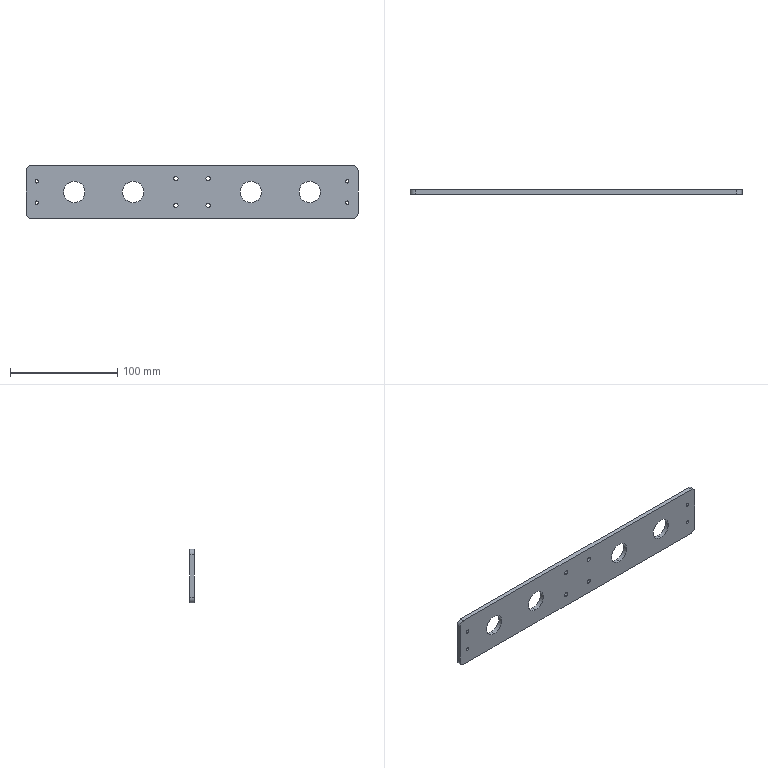Part | SolidWorks | features BaseBody 1 | 1 solid | 34 faces | box 310 x 4 x 50 mm | volume 56558 mm3 | cylinder 28 | plane 6 | commonest cylinder face diameters 3.2 x8 4 x8 20 x8 10 x4
STEP:
#1=CARTESIAN_POINT('',(15.,4.,-10.5));
#2=VERTEX_POINT('',#1);
#3=CARTESIAN_POINT('',(15.,4.,-14.5));
#4=VERTEX_POINT('',#3);
#5=CARTESIAN_POINT('',(15.,4.,-12.5));
#6=DIRECTION('',(0.,-1.,0.));
#7=DIRECTION('',(0.,0.,-1.));
#8=AXIS2_PLACEMENT_3D('',#5,#6,#7);
#9=CIRCLE('',#8,2.);
#10=EDGE_CURVE('',#2,#4,#9,.T.);
#11=ORIENTED_EDGE('',*,*,#10,.F.);
#12=CARTESIAN_POINT('',(15.,0.,-10.5));
#13=VERTEX_POINT('',#12);
#14=CARTESIAN_POINT('',(15.,4.,-10.5));
#15=DIRECTION('',(0.,-1.,0.));
#16=VECTOR('',#15,1000.);
#17=LINE('',#14,#16);
#18=EDGE_CURVE('',#2,#13,#17,.T.);
#19=ORIENTED_EDGE('',*,*,#18,.T.);
#20=CARTESIAN_POINT('',(15.,0.,-14.5));
#21=VERTEX_POINT('',#20);
#22=CARTESIAN_POINT('',(15.,0.,-12.5));
#23=DIRECTION('',(0.,-1.,0.));
#24=DIRECTION('',(0.,0.,-1.));
#25=AXIS2_PLACEMENT_3D('',#22,#23,#24);
#26=CIRCLE('',#25,2.);
#27=EDGE_CURVE('',#13,#21,#26,.T.);
#28=ORIENTED_EDGE('',*,*,#27,.T.);
#29=CARTESIAN_POINT('',(15.,4.,-14.5));
#30=DIRECTION('',(0.,-1.,0.));
#31=VECTOR('',#30,1000.);
#32=LINE('',#29,#31);
#33=EDGE_CURVE('',#4,#21,#32,.T.);
#34=ORIENTED_EDGE('',*,*,#33,.F.);
#35=EDGE_LOOP('',(#11,#19,#28,#34));
#36=FACE_OUTER_BOUND('',#35,.T.);
#37=CARTESIAN_POINT('',(15.,4.,-12.5));
#38=DIRECTION('',(0.,-1.,0.));
#39=DIRECTION('',(0.,0.,-1.));
#40=AXIS2_PLACEMENT_3D('',#37,#38,#39);
#41=CYLINDRICAL_SURFACE('',#40,2.);
#42=ADVANCED_FACE('',(#36),#41,.F.);
#43=CARTESIAN_POINT('',(15.,4.,14.5));
#44=VERTEX_POINT('',#43);
#45=CARTESIAN_POINT('',(15.,4.,10.5));
#46=VERTEX_POINT('',#45);
#47=CARTESIAN_POINT('',(15.,4.,12.5));
#48=DIRECTION('',(0.,-1.,0.));
#49=DIRECTION('',(0.,0.,-1.));
#50=AXIS2_PLACEMENT_3D('',#47,#48,#49);
#51=CIRCLE('',#50,2.);
#52=EDGE_CURVE('',#44,#46,#51,.T.);
#53=ORIENTED_EDGE('',*,*,#52,.F.);
#54=CARTESIAN_POINT('',(15.,0.,14.5));
#55=VERTEX_POINT('',#54);
#56=CARTESIAN_POINT('',(15.,4.,14.5));
#57=DIRECTION('',(0.,-1.,0.));
#58=VECTOR('',#57,1000.);
#59=LINE('',#56,#58);
#60=EDGE_CURVE('',#44,#55,#59,.T.);
#61=ORIENTED_EDGE('',*,*,#60,.T.);
#62=CARTESIAN_POINT('',(15.,0.,10.5));
#63=VERTEX_POINT('',#62);
#64=CARTESIAN_POINT('',(15.,0.,12.5));
#65=DIRECTION('',(0.,-1.,0.));
#66=DIRECTION('',(0.,0.,-1.));
#67=AXIS2_PLACEMENT_3D('',#64,#65,#66);
#68=CIRCLE('',#67,2.);
#69=EDGE_CURVE('',#55,#63,#68,.T.);
#70=ORIENTED_EDGE('',*,*,#69,.T.);
#71=CARTESIAN_POINT('',(15.,4.,10.5));
#72=DIRECTION('',(0.,-1.,0.));
#73=VECTOR('',#72,1000.);
#74=LINE('',#71,#73);
#75=EDGE_CURVE('',#46,#63,#74,.T.);
#76=ORIENTED_EDGE('',*,*,#75,.F.);
#77=EDGE_LOOP('',(#53,#61,#70,#76));
#78=FACE_OUTER_BOUND('',#77,.T.);
#79=CARTESIAN_POINT('',(15.,4.,12.5));
#80=DIRECTION('',(0.,-1.,0.));
#81=DIRECTION('',(0.,0.,-1.));
#82=AXIS2_PLACEMENT_3D('',#79,#80,#81);
#83=CYLINDRICAL_SURFACE('',#82,2.);
#84=ADVANCED_FACE('',(#78),#83,.F.);
#85=CARTESIAN_POINT('',(-15.,4.,14.5));
#86=VERTEX_POINT('',#85);
#87=CARTESIAN_POINT('',(-15.,4.,10.5));
#88=VERTEX_POINT('',#87);
#89=CARTESIAN_POINT('',(-15.,4.,12.5));
#90=DIRECTION('',(0.,-1.,0.));
#91=DIRECTION('',(0.,0.,-1.));
#92=AXIS2_PLACEMENT_3D('',#89,#90,#91);
#93=CIRCLE('',#92,2.);
#94=EDGE_CURVE('',#86,#88,#93,.T.);
#95=ORIENTED_EDGE('',*,*,#94,.F.);
#96=CARTESIAN_POINT('',(-15.,0.,14.5));
#97=VERTEX_POINT('',#96);
#98=CARTESIAN_POINT('',(-15.,4.,14.5));
#99=DIRECTION('',(0.,-1.,0.));
#100=VECTOR('',#99,1000.);
#101=LINE('',#98,#100);
#102=EDGE_CURVE('',#86,#97,#101,.T.);
#103=ORIENTED_EDGE('',*,*,#102,.T.);
#104=CARTESIAN_POINT('',(-15.,0.,10.5));
#105=VERTEX_POINT('',#104);
#106=CARTESIAN_POINT('',(-15.,0.,12.5));
#107=DIRECTION('',(0.,-1.,0.));
#108=DIRECTION('',(0.,0.,-1.));
#109=AXIS2_PLACEMENT_3D('',#106,#107,#108);
#110=CIRCLE('',#109,2.);
#111=EDGE_CURVE('',#97,#105,#110,.T.);
#112=ORIENTED_EDGE('',*,*,#111,.T.);
#113=CARTESIAN_POINT('',(-15.,4.,10.5));
#114=DIRECTION('',(0.,-1.,0.));
#115=VECTOR('',#114,1000.);
#116=LINE('',#113,#115);
#117=EDGE_CURVE('',#88,#105,#116,.T.);
#118=ORIENTED_EDGE('',*,*,#117,.F.);
#119=EDGE_LOOP('',(#95,#103,#112,#118));
#120=FACE_OUTER_BOUND('',#119,.T.);
#121=CARTESIAN_POINT('',(-15.,4.,12.5));
#122=DIRECTION('',(0.,-1.,0.));
#123=DIRECTION('',(0.,0.,-1.));
#124=AXIS2_PLACEMENT_3D('',#121,#122,#123);
#125=CYLINDRICAL_SURFACE('',#124,2.);
#126=ADVANCED_FACE('',(#120),#125,.F.);
#127=CARTESIAN_POINT('',(-15.,4.,-10.5));
#128=VERTEX_POINT('',#127);
#129=CARTESIAN_POINT('',(-15.,4.,-14.5));
#130=VERTEX_POINT('',#129);
#131=CARTESIAN_POINT('',(-15.,4.,-12.5));
#132=DIRECTION('',(0.,-1.,0.));
#133=DIRECTION('',(0.,0.,-1.));
#134=AXIS2_PLACEMENT_3D('',#131,#132,#133);
#135=CIRCLE('',#134,2.);
#136=EDGE_CURVE('',#128,#130,#135,.T.);
#137=ORIENTED_EDGE('',*,*,#136,.F.);
#138=CARTESIAN_POINT('',(-15.,0.,-10.5));
#139=VERTEX_POINT('',#138);
#140=CARTESIAN_POINT('',(-15.,4.,-10.5));
#141=DIRECTION('',(0.,-1.,0.));
#142=VECTOR('',#141,1000.);
#143=LINE('',#140,#142);
#144=EDGE_CURVE('',#128,#139,#143,.T.);
#145=ORIENTED_EDGE('',*,*,#144,.T.);
#146=CARTESIAN_POINT('',(-15.,0.,-14.5));
#147=VERTEX_POINT('',#146);
#148=CARTESIAN_POINT('',(-15.,0.,-12.5));
#149=DIRECTION('',(0.,-1.,0.));
#150=DIRECTION('',(0.,0.,-1.));
#151=AXIS2_PLACEMENT_3D('',#148,#149,#150);
#152=CIRCLE('',#151,2.);
#153=EDGE_CURVE('',#139,#147,#152,.T.);
#154=ORIENTED_EDGE('',*,*,#153,.T.);
#155=CARTESIAN_POINT('',(-15.,4.,-14.5));
#156=DIRECTION('',(0.,-1.,0.));
#157=VECTOR('',#156,1000.);
#158=LINE('',#155,#157);
#159=EDGE_CURVE('',#130,#147,#158,.T.);
#160=ORIENTED_EDGE('',*,*,#159,.F.);
#161=EDGE_LOOP('',(#137,#145,#154,#160));
#162=FACE_OUTER_BOUND('',#161,.T.);
#163=CARTESIAN_POINT('',(-15.,4.,-12.5));
#164=DIRECTION('',(0.,-1.,0.));
#165=DIRECTION('',(0.,0.,-1.));
#166=AXIS2_PLACEMENT_3D('',#163,#164,#165);
#167=CYLINDRICAL_SURFACE('',#166,2.);
#168=ADVANCED_FACE('',(#162),#167,.F.);
#169=CARTESIAN_POINT('',(-145.,4.,11.6));
#170=VERTEX_POINT('',#169);
#171=CARTESIAN_POINT('',(-145.,4.,8.4));
#172=VERTEX_POINT('',#171);
#173=CARTESIAN_POINT('',(-145.,4.,10.));
#174=DIRECTION('',(0.,-1.,0.));
#175=DIRECTION('',(0.,0.,-1.));
#176=AXIS2_PLACEMENT_3D('',#173,#174,#175);
#177=CIRCLE('',#176,1.6);
#178=EDGE_CURVE('',#170,#172,#177,.T.);
#179=ORIENTED_EDGE('',*,*,#178,.F.);
#180=CARTESIAN_POINT('',(-145.,0.,11.6));
#181=VERTEX_POINT('',#180);
#182=CARTESIAN_POINT('',(-145.,20.,11.6));
#183=DIRECTION('',(0.,-1.,0.));
#184=VECTOR('',#183,1000.);
#185=LINE('',#182,#184);
#186=EDGE_CURVE('',#170,#181,#185,.T.);
#187=ORIENTED_EDGE('',*,*,#186,.T.);
#188=CARTESIAN_POINT('',(-145.,0.,8.4));
#189=VERTEX_POINT('',#188);
#190=CARTESIAN_POINT('',(-145.,0.,10.));
#191=DIRECTION('',(0.,-1.,0.));
#192=DIRECTION('',(0.,0.,-1.));
#193=AXIS2_PLACEMENT_3D('',#190,#191,#192);
#194=CIRCLE('',#193,1.6);
#195=EDGE_CURVE('',#181,#189,#194,.T.);
#196=ORIENTED_EDGE('',*,*,#195,.T.);
#197=CARTESIAN_POINT('',(-145.,20.,8.4));
#198=DIRECTION('',(0.,-1.,0.));
#199=VECTOR('',#198,1000.);
#200=LINE('',#197,#199);
#201=EDGE_CURVE('',#172,#189,#200,.T.);
#202=ORIENTED_EDGE('',*,*,#201,.F.);
#203=EDGE_LOOP('',(#179,#187,#196,#202));
#204=FACE_OUTER_BOUND('',#203,.T.);
#205=CARTESIAN_POINT('',(-145.,20.,10.));
#206=DIRECTION('',(0.,-1.,0.));
#207=DIRECTION('',(0.,0.,-1.));
#208=AXIS2_PLACEMENT_3D('',#205,#206,#207);
#209=CYLINDRICAL_SURFACE('',#208,1.6);
#210=ADVANCED_FACE('',(#204),#209,.F.);
#211=CARTESIAN_POINT('',(-145.,4.,-8.4));
#212=VERTEX_POINT('',#211);
#213=CARTESIAN_POINT('',(-145.,4.,-11.6));
#214=VERTEX_POINT('',#213);
#215=CARTESIAN_POINT('',(-145.,4.,-10.));
#216=DIRECTION('',(0.,-1.,0.));
#217=DIRECTION('',(0.,0.,-1.));
#218=AXIS2_PLACEMENT_3D('',#215,#216,#217);
#219=CIRCLE('',#218,1.6);
#220=EDGE_CURVE('',#212,#214,#219,.T.);
#221=ORIENTED_EDGE('',*,*,#220,.F.);
#222=CARTESIAN_POINT('',(-145.,0.,-8.4));
#223=VERTEX_POINT('',#222);
#224=CARTESIAN_POINT('',(-145.,20.,-8.4));
#225=DIRECTION('',(0.,-1.,0.));
#226=VECTOR('',#225,1000.);
#227=LINE('',#224,#226);
#228=EDGE_CURVE('',#212,#223,#227,.T.);
#229=ORIENTED_EDGE('',*,*,#228,.T.);
#230=CARTESIAN_POINT('',(-145.,0.,-11.6));
#231=VERTEX_POINT('',#230);
#232=CARTESIAN_POINT('',(-145.,0.,-10.));
#233=DIRECTION('',(0.,-1.,0.));
#234=DIRECTION('',(0.,0.,-1.));
#235=AXIS2_PLACEMENT_3D('',#232,#233,#234);
#236=CIRCLE('',#235,1.6);
#237=EDGE_CURVE('',#223,#231,#236,.T.);
#238=ORIENTED_EDGE('',*,*,#237,.T.);
#239=CARTESIAN_POINT('',(-145.,20.,-11.6));
#240=DIRECTION('',(0.,-1.,0.));
#241=VECTOR('',#240,1000.);
#242=LINE('',#239,#241);
#243=EDGE_CURVE('',#214,#231,#242,.T.);
#244=ORIENTED_EDGE('',*,*,#243,.F.);
#245=EDGE_LOOP('',(#221,#229,#238,#244));
#246=FACE_OUTER_BOUND('',#245,.T.);
#247=CARTESIAN_POINT('',(-145.,20.,-10.));
#248=DIRECTION('',(0.,-1.,0.));
#249=DIRECTION('',(0.,0.,-1.));
#250=AXIS2_PLACEMENT_3D('',#247,#248,#249);
#251=CYLINDRICAL_SURFACE('',#250,1.6);
#252=ADVANCED_FACE('',(#246),#251,.F.);
#253=CARTESIAN_POINT('',(145.,4.,-8.4));
#254=VERTEX_POINT('',#253);
#255=CARTESIAN_POINT('',(145.,4.,-11.6));
#256=VERTEX_POINT('',#255);
#257=CARTESIAN_POINT('',(145.,4.,-10.));
#258=DIRECTION('',(0.,-1.,0.));
#259=DIRECTION('',(0.,0.,-1.));
#260=AXIS2_PLACEMENT_3D('',#257,#258,#259);
#261=CIRCLE('',#260,1.6);
#262=EDGE_CURVE('',#254,#256,#261,.T.);
#263=ORIENTED_EDGE('',*,*,#262,.F.);
#264=CARTESIAN_POINT('',(145.,0.,-8.4));
#265=VERTEX_POINT('',#264);
#266=CARTESIAN_POINT('',(145.,20.,-8.4));
#267=DIRECTION('',(0.,-1.,0.));
#268=VECTOR('',#267,1000.);
#269=LINE('',#266,#268);
#270=EDGE_CURVE('',#254,#265,#269,.T.);
#271=ORIENTED_EDGE('',*,*,#270,.T.);
#272=CARTESIAN_POINT('',(145.,0.,-11.6));
#273=VERTEX_POINT('',#272);
#274=CARTESIAN_POINT('',(145.,0.,-10.));
#275=DIRECTION('',(0.,-1.,0.));
#276=DIRECTION('',(0.,0.,-1.));
#277=AXIS2_PLACEMENT_3D('',#274,#275,#276);
#278=CIRCLE('',#277,1.6);
#279=EDGE_CURVE('',#265,#273,#278,.T.);
#280=ORIENTED_EDGE('',*,*,#279,.T.);
#281=CARTESIAN_POINT('',(145.,20.,-11.6));
#282=DIRECTION('',(0.,-1.,0.));
#283=VECTOR('',#282,1000.);
#284=LINE('',#281,#283);
#285=EDGE_CURVE('',#256,#273,#284,.T.);
#286=ORIENTED_EDGE('',*,*,#285,.F.);
#287=EDGE_LOOP('',(#263,#271,#280,#286));
#288=FACE_OUTER_BOUND('',#287,.T.);
#289=CARTESIAN_POINT('',(145.,20.,-10.));
#290=DIRECTION('',(0.,-1.,0.));
#291=DIRECTION('',(0.,0.,-1.));
#292=AXIS2_PLACEMENT_3D('',#289,#290,#291);
#293=CYLINDRICAL_SURFACE('',#292,1.6);
#294=ADVANCED_FACE('',(#288),#293,.F.);
#295=CARTESIAN_POINT('',(145.,4.,11.6));
#296=VERTEX_POINT('',#295);
#297=CARTESIAN_POINT('',(145.,4.,8.4));
#298=VERTEX_POINT('',#297);
#299=CARTESIAN_POINT('',(145.,4.,10.));
#300=DIRECTION('',(0.,-1.,0.));
#301=DIRECTION('',(0.,0.,-1.));
#302=AXIS2_PLACEMENT_3D('',#299,#300,#301);
#303=CIRCLE('',#302,1.6);
#304=EDGE_CURVE('',#296,#298,#303,.T.);
#305=ORIENTED_EDGE('',*,*,#304,.F.);
#306=CARTESIAN_POINT('',(145.,0.,11.6));
#307=VERTEX_POINT('',#306);
#308=CARTESIAN_POINT('',(145.,20.,11.6));
#309=DIRECTION('',(0.,-1.,0.));
#310=VECTOR('',#309,1000.);
#311=LINE('',#308,#310);
#312=EDGE_CURVE('',#296,#307,#311,.T.);
#313=ORIENTED_EDGE('',*,*,#312,.T.);
#314=CARTESIAN_POINT('',(145.,0.,8.4));
#315=VERTEX_POINT('',#314);
#316=CARTESIAN_POINT('',(145.,0.,10.));
#317=DIRECTION('',(0.,-1.,0.));
#318=DIRECTION('',(0.,0.,-1.));
#319=AXIS2_PLACEMENT_3D('',#316,#317,#318);
#320=CIRCLE('',#319,1.6);
#321=EDGE_CURVE('',#307,#315,#320,.T.);
#322=ORIENTED_EDGE('',*,*,#321,.T.);
#323=CARTESIAN_POINT('',(145.,20.,8.4));
#324=DIRECTION('',(0.,-1.,0.));
#325=VECTOR('',#324,1000.);
#326=LINE('',#323,#325);
#327=EDGE_CURVE('',#298,#315,#326,.T.);
#328=ORIENTED_EDGE('',*,*,#327,.F.);
#329=EDGE_LOOP('',(#305,#313,#322,#328));
#330=FACE_OUTER_BOUND('',#329,.T.);
#331=CARTESIAN_POINT('',(145.,20.,10.));
#332=DIRECTION('',(0.,-1.,0.));
#333=DIRECTION('',(0.,0.,-1.));
#334=AXIS2_PLACEMENT_3D('',#331,#332,#333);
#335=CYLINDRICAL_SURFACE('',#334,1.6);
#336=ADVANCED_FACE('',(#330),#335,.F.);
#337=CARTESIAN_POINT('',(110.,4.,10.));
#338=VERTEX_POINT('',#337);
#339=CARTESIAN_POINT('',(110.,4.,-10.));
#340=VERTEX_POINT('',#339);
#341=CARTESIAN_POINT('',(110.,4.,0.));
#342=DIRECTION('',(0.,-1.,0.));
#343=DIRECTION('',(0.,0.,-1.));
#344=AXIS2_PLACEMENT_3D('',#341,#342,#343);
#345=CIRCLE('',#344,10.);
#346=EDGE_CURVE('',#338,#340,#345,.T.);
#347=ORIENTED_EDGE('',*,*,#346,.F.);
#348=CARTESIAN_POINT('',(110.,0.,10.));
#349=VERTEX_POINT('',#348);
#350=CARTESIAN_POINT('',(110.,20.,10.));
#351=DIRECTION('',(0.,-1.,0.));
#352=VECTOR('',#351,1000.);
#353=LINE('',#350,#352);
#354=EDGE_CURVE('',#338,#349,#353,.T.);
#355=ORIENTED_EDGE('',*,*,#354,.T.);
#356=CARTESIAN_POINT('',(110.,0.,-10.));
#357=VERTEX_POINT('',#356);
#358=CARTESIAN_POINT('',(110.,0.,0.));
#359=DIRECTION('',(0.,-1.,0.));
#360=DIRECTION('',(0.,0.,-1.));
#361=AXIS2_PLACEMENT_3D('',#358,#359,#360);
#362=CIRCLE('',#361,10.);
#363=EDGE_CURVE('',#349,#357,#362,.T.);
#364=ORIENTED_EDGE('',*,*,#363,.T.);
#365=CARTESIAN_POINT('',(110.,20.,-10.));
#366=DIRECTION('',(0.,-1.,0.));
#367=VECTOR('',#366,1000.);
#368=LINE('',#365,#367);
#369=EDGE_CURVE('',#340,#357,#368,.T.);
#370=ORIENTED_EDGE('',*,*,#369,.F.);
#371=EDGE_LOOP('',(#347,#355,#364,#370));
#372=FACE_OUTER_BOUND('',#371,.T.);
#373=CARTESIAN_POINT('',(110.,20.,0.));
#374=DIRECTION('',(0.,-1.,0.));
#375=DIRECTION('',(0.,0.,-1.));
#376=AXIS2_PLACEMENT_3D('',#373,#374,#375);
#377=CYLINDRICAL_SURFACE('',#376,10.);
#378=ADVANCED_FACE('',(#372),#377,.F.);
#379=CARTESIAN_POINT('',(55.,4.,10.));
#380=VERTEX_POINT('',#379);
#381=CARTESIAN_POINT('',(55.,4.,-10.));
#382=VERTEX_POINT('',#381);
#383=CARTESIAN_POINT('',(55.,4.,0.));
#384=DIRECTION('',(0.,-1.,0.));
#385=DIRECTION('',(0.,0.,-1.));
#386=AXIS2_PLACEMENT_3D('',#383,#384,#385);
#387=CIRCLE('',#386,10.);
#388=EDGE_CURVE('',#380,#382,#387,.T.);
#389=ORIENTED_EDGE('',*,*,#388,.F.);
#390=CARTESIAN_POINT('',(55.,0.,10.));
#391=VERTEX_POINT('',#390);
#392=CARTESIAN_POINT('',(55.,20.,10.));
#393=DIRECTION('',(0.,-1.,0.));
#394=VECTOR('',#393,1000.);
#395=LINE('',#392,#394);
#396=EDGE_CURVE('',#380,#391,#395,.T.);
#397=ORIENTED_EDGE('',*,*,#396,.T.);
#398=CARTESIAN_POINT('',(55.,0.,-10.));
#399=VERTEX_POINT('',#398);
#400=CARTESIAN_POINT('',(55.,0.,0.));
#401=DIRECTION('',(0.,-1.,0.));
#402=DIRECTION('',(0.,0.,-1.));
#403=AXIS2_PLACEMENT_3D('',#400,#401,#402);
#404=CIRCLE('',#403,10.);
#405=EDGE_CURVE('',#391,#399,#404,.T.);
#406=ORIENTED_EDGE('',*,*,#405,.T.);
#407=CARTESIAN_POINT('',(55.,20.,-10.));
#408=DIRECTION('',(0.,-1.,0.));
#409=VECTOR('',#408,1000.);
#410=LINE('',#407,#409);
#411=EDGE_CURVE('',#382,#399,#410,.T.);
#412=ORIENTED_EDGE('',*,*,#411,.F.);
#413=EDGE_LOOP('',(#389,#397,#406,#412));
#414=FACE_OUTER_BOUND('',#413,.T.);
#415=CARTESIAN_POINT('',(55.,20.,0.));
#416=DIRECTION('',(0.,-1.,0.));
#417=DIRECTION('',(0.,0.,-1.));
#418=AXIS2_PLACEMENT_3D('',#415,#416,#417);
#419=CYLINDRICAL_SURFACE('',#418,10.);
#420=ADVANCED_FACE('',(#414),#419,.F.);
#421=CARTESIAN_POINT('',(-55.,4.,10.));
#422=VERTEX_POINT('',#421);
#423=CARTESIAN_POINT('',(-55.,4.,-10.));
#424=VERTEX_POINT('',#423);
#425=CARTESIAN_POINT('',(-55.,4.,0.));
#426=DIRECTION('',(0.,-1.,0.));
#427=DIRECTION('',(0.,0.,-1.));
#428=AXIS2_PLACEMENT_3D('',#425,#426,#427);
#429=CIRCLE('',#428,10.);
#430=EDGE_CURVE('',#422,#424,#429,.T.);
#431=ORIENTED_EDGE('',*,*,#430,.F.);
#432=CARTESIAN_POINT('',(-55.,0.,10.));
#433=VERTEX_POINT('',#432);
#434=CARTESIAN_POINT('',(-55.,20.,10.));
#435=DIRECTION('',(0.,-1.,0.));
#436=VECTOR('',#435,1000.);
#437=LINE('',#434,#436);
#438=EDGE_CURVE('',#422,#433,#437,.T.);
#439=ORIENTED_EDGE('',*,*,#438,.T.);
#440=CARTESIAN_POINT('',(-55.,0.,-10.));
#441=VERTEX_POINT('',#440);
#442=CARTESIAN_POINT('',(-55.,0.,0.));
#443=DIRECTION('',(0.,-1.,0.));
#444=DIRECTION('',(0.,0.,-1.));
#445=AXIS2_PLACEMENT_3D('',#442,#443,#444);
#446=CIRCLE('',#445,10.);
#447=EDGE_CURVE('',#433,#441,#446,.T.);
#448=ORIENTED_EDGE('',*,*,#447,.T.);
#449=CARTESIAN_POINT('',(-55.,20.,-10.));
#450=DIRECTION('',(0.,-1.,0.));
#451=VECTOR('',#450,1000.);
#452=LINE('',#449,#451);
#453=EDGE_CURVE('',#424,#441,#452,.T.);
#454=ORIENTED_EDGE('',*,*,#453,.F.);
#455=EDGE_LOOP('',(#431,#439,#448,#454));
#456=FACE_OUTER_BOUND('',#455,.T.);
#457=CARTESIAN_POINT('',(-55.,20.,0.));
#458=DIRECTION('',(0.,-1.,0.));
#459=DIRECTION('',(0.,0.,-1.));
#460=AXIS2_PLACEMENT_3D('',#457,#458,#459);
#461=CYLINDRICAL_SURFACE('',#460,10.);
#462=ADVANCED_FACE('',(#456),#461,.F.);
#463=CARTESIAN_POINT('',(-110.,4.,10.));
#464=VERTEX_POINT('',#463);
#465=CARTESIAN_POINT('',(-110.,4.,-10.));
#466=VERTEX_POINT('',#465);
#467=CARTESIAN_POINT('',(-110.,4.,0.));
#468=DIRECTION('',(0.,-1.,0.));
#469=DIRECTION('',(0.,0.,-1.));
#470=AXIS2_PLACEMENT_3D('',#467,#468,#469);
#471=CIRCLE('',#470,10.);
#472=EDGE_CURVE('',#464,#466,#471,.T.);
#473=ORIENTED_EDGE('',*,*,#472,.F.);
#474=CARTESIAN_POINT('',(-110.,0.,10.));
#475=VERTEX_POINT('',#474);
#476=CARTESIAN_POINT('',(-110.,20.,10.));
#477=DIRECTION('',(0.,-1.,0.));
#478=VECTOR('',#477,1000.);
#479=LINE('',#476,#478);
#480=EDGE_CURVE('',#464,#475,#479,.T.);
#481=ORIENTED_EDGE('',*,*,#480,.T.);
#482=CARTESIAN_POINT('',(-110.,0.,-10.));
#483=VERTEX_POINT('',#482);
#484=CARTESIAN_POINT('',(-110.,0.,0.));
#485=DIRECTION('',(0.,-1.,0.));
#486=DIRECTION('',(0.,0.,-1.));
#487=AXIS2_PLACEMENT_3D('',#484,#485,#486);
#488=CIRCLE('',#487,10.);
#489=EDGE_CURVE('',#475,#483,#488,.T.);
#490=ORIENTED_EDGE('',*,*,#489,.T.);
#491=CARTESIAN_POINT('',(-110.,20.,-10.));
#492=DIRECTION('',(0.,-1.,0.));
#493=VECTOR('',#492,1000.);
#494=LINE('',#491,#493);
#495=EDGE_CURVE('',#466,#483,#494,.T.);
#496=ORIENTED_EDGE('',*,*,#495,.F.);
#497=EDGE_LOOP('',(#473,#481,#490,#496));
#498=FACE_OUTER_BOUND('',#497,.T.);
#499=CARTESIAN_POINT('',(-110.,20.,0.));
#500=DIRECTION('',(0.,-1.,0.));
#501=DIRECTION('',(0.,0.,-1.));
#502=AXIS2_PLACEMENT_3D('',#499,#500,#501);
#503=CYLINDRICAL_SURFACE('',#502,10.);
#504=ADVANCED_FACE('',(#498),#503,.F.);
#505=CARTESIAN_POINT('',(15.,0.,-12.5));
#506=DIRECTION('',(0.,-1.,0.));
#507=DIRECTION('',(0.,0.,-1.));
#508=AXIS2_PLACEMENT_3D('',#505,#506,#507);
#509=CIRCLE('',#508,2.);
#510=EDGE_CURVE('',#21,#13,#509,.T.);
#511=ORIENTED_EDGE('',*,*,#510,.F.);
#512=ORIENTED_EDGE('',*,*,#27,.F.);
#513=EDGE_LOOP('',(#511,#512));
#514=FACE_BOUND('',#513,.T.);
#515=CARTESIAN_POINT('',(15.,0.,12.5));
#516=DIRECTION('',(0.,-1.,0.));
#517=DIRECTION('',(0.,0.,-1.));
#518=AXIS2_PLACEMENT_3D('',#515,#516,#517);
#519=CIRCLE('',#518,2.);
#520=EDGE_CURVE('',#63,#55,#519,.T.);
#521=ORIENTED_EDGE('',*,*,#520,.F.);
#522=ORIENTED_EDGE('',*,*,#69,.F.);
#523=EDGE_LOOP('',(#521,#522));
#524=FACE_BOUND('',#523,.T.);
#525=CARTESIAN_POINT('',(-15.,0.,12.5));
#526=DIRECTION('',(0.,-1.,0.));
#527=DIRECTION('',(0.,0.,-1.));
#528=AXIS2_PLACEMENT_3D('',#525,#526,#527);
#529=CIRCLE('',#528,2.);
#530=EDGE_CURVE('',#105,#97,#529,.T.);
#531=ORIENTED_EDGE('',*,*,#530,.F.);
#532=ORIENTED_EDGE('',*,*,#111,.F.);
#533=EDGE_LOOP('',(#531,#532));
#534=FACE_BOUND('',#533,.T.);
#535=CARTESIAN_POINT('',(-15.,0.,-12.5));
#536=DIRECTION('',(0.,-1.,0.));
#537=DIRECTION('',(0.,0.,-1.));
#538=AXIS2_PLACEMENT_3D('',#535,#536,#537);
#539=CIRCLE('',#538,2.);
#540=EDGE_CURVE('',#147,#139,#539,.T.);
#541=ORIENTED_EDGE('',*,*,#540,.F.);
#542=ORIENTED_EDGE('',*,*,#153,.F.);
#543=EDGE_LOOP('',(#541,#542));
#544=FACE_BOUND('',#543,.T.);
#545=CARTESIAN_POINT('',(155.,0.,-20.));
#546=VERTEX_POINT('',#545);
#547=CARTESIAN_POINT('',(150.,0.,-25.));
#548=VERTEX_POINT('',#547);
#549=CARTESIAN_POINT('',(150.,0.,-20.));
#550=DIRECTION('',(0.,1.,0.));
#551=DIRECTION('',(0.,0.,-1.));
#552=AXIS2_PLACEMENT_3D('',#549,#550,#551);
#553=CIRCLE('',#552,5.);
#554=EDGE_CURVE('',#546,#548,#553,.T.);
#555=ORIENTED_EDGE('',*,*,#554,.F.);
#556=CARTESIAN_POINT('',(155.,0.,20.));
#557=VERTEX_POINT('',#556);
#558=CARTESIAN_POINT('',(155.,0.,0.));
#559=DIRECTION('',(0.,0.,-1.));
#560=VECTOR('',#559,1000.);
#561=LINE('',#558,#560);
#562=EDGE_CURVE('',#557,#546,#561,.T.);
#563=ORIENTED_EDGE('',*,*,#562,.F.);
#564=CARTESIAN_POINT('',(150.,0.,25.));
#565=VERTEX_POINT('',#564);
#566=CARTESIAN_POINT('',(150.,0.,20.));
#567=DIRECTION('',(0.,1.,0.));
#568=DIRECTION('',(0.,0.,-1.));
#569=AXIS2_PLACEMENT_3D('',#566,#567,#568);
#570=CIRCLE('',#569,5.);
#571=EDGE_CURVE('',#565,#557,#570,.T.);
#572=ORIENTED_EDGE('',*,*,#571,.F.);
#573=CARTESIAN_POINT('',(-150.,0.,25.));
#574=VERTEX_POINT('',#573);
#575=CARTESIAN_POINT('',(0.,0.,25.));
#576=DIRECTION('',(1.,0.,0.));
#577=VECTOR('',#576,1000.);
#578=LINE('',#575,#577);
#579=EDGE_CURVE('',#574,#565,#578,.T.);
#580=ORIENTED_EDGE('',*,*,#579,.F.);
#581=CARTESIAN_POINT('',(-155.,0.,20.));
#582=VERTEX_POINT('',#581);
#583=CARTESIAN_POINT('',(-150.,0.,20.));
#584=DIRECTION('',(0.,1.,0.));
#585=DIRECTION('',(0.,0.,-1.));
#586=AXIS2_PLACEMENT_3D('',#583,#584,#585);
#587=CIRCLE('',#586,5.);
#588=EDGE_CURVE('',#582,#574,#587,.T.);
#589=ORIENTED_EDGE('',*,*,#588,.F.);
#590=CARTESIAN_POINT('',(-155.,0.,-20.));
#591=VERTEX_POINT('',#590);
#592=CARTESIAN_POINT('',(-155.,0.,0.));
#593=DIRECTION('',(0.,0.,1.));
#594=VECTOR('',#593,1000.);
#595=LINE('',#592,#594);
#596=EDGE_CURVE('',#591,#582,#595,.T.);
#597=ORIENTED_EDGE('',*,*,#596,.F.);
#598=CARTESIAN_POINT('',(-150.,0.,-25.));
#599=VERTEX_POINT('',#598);
#600=CARTESIAN_POINT('',(-150.,0.,-20.));
#601=DIRECTION('',(0.,1.,0.));
#602=DIRECTION('',(0.,0.,-1.));
#603=AXIS2_PLACEMENT_3D('',#600,#601,#602);
#604=CIRCLE('',#603,5.);
#605=EDGE_CURVE('',#599,#591,#604,.T.);
#606=ORIENTED_EDGE('',*,*,#605,.F.);
#607=CARTESIAN_POINT('',(0.,0.,-25.));
#608=DIRECTION('',(-1.,0.,0.));
#609=VECTOR('',#608,1000.);
#610=LINE('',#607,#609);
#611=EDGE_CURVE('',#548,#599,#610,.T.);
#612=ORIENTED_EDGE('',*,*,#611,.F.);
#613=EDGE_LOOP('',(#555,#563,#572,#580,#589,#597,#606,#612));
#614=FACE_OUTER_BOUND('',#613,.T.);
#615=CARTESIAN_POINT('',(-145.,0.,10.));
#616=DIRECTION('',(0.,-1.,0.));
#617=DIRECTION('',(0.,0.,-1.));
#618=AXIS2_PLACEMENT_3D('',#615,#616,#617);
#619=CIRCLE('',#618,1.6);
#620=EDGE_CURVE('',#189,#181,#619,.T.);
#621=ORIENTED_EDGE('',*,*,#620,.F.);
#622=ORIENTED_EDGE('',*,*,#195,.F.);
#623=EDGE_LOOP('',(#621,#622));
#624=FACE_BOUND('',#623,.T.);
#625=CARTESIAN_POINT('',(-145.,0.,-10.));
#626=DIRECTION('',(0.,-1.,0.));
#627=DIRECTION('',(0.,0.,-1.));
#628=AXIS2_PLACEMENT_3D('',#625,#626,#627);
#629=CIRCLE('',#628,1.6);
#630=EDGE_CURVE('',#231,#223,#629,.T.);
#631=ORIENTED_EDGE('',*,*,#630,.F.);
#632=ORIENTED_EDGE('',*,*,#237,.F.);
#633=EDGE_LOOP('',(#631,#632));
#634=FACE_BOUND('',#633,.T.);
#635=CARTESIAN_POINT('',(145.,0.,-10.));
#636=DIRECTION('',(0.,-1.,0.));
#637=DIRECTION('',(0.,0.,-1.));
#638=AXIS2_PLACEMENT_3D('',#635,#636,#637);
#639=CIRCLE('',#638,1.6);
#640=EDGE_CURVE('',#273,#265,#639,.T.);
#641=ORIENTED_EDGE('',*,*,#640,.F.);
#642=ORIENTED_EDGE('',*,*,#279,.F.);
#643=EDGE_LOOP('',(#641,#642));
#644=FACE_BOUND('',#643,.T.);
#645=CARTESIAN_POINT('',(145.,0.,10.));
#646=DIRECTION('',(0.,-1.,0.));
#647=DIRECTION('',(0.,0.,-1.));
#648=AXIS2_PLACEMENT_3D('',#645,#646,#647);
#649=CIRCLE('',#648,1.6);
#650=EDGE_CURVE('',#315,#307,#649,.T.);
#651=ORIENTED_EDGE('',*,*,#650,.F.);
#652=ORIENTED_EDGE('',*,*,#321,.F.);
#653=EDGE_LOOP('',(#651,#652));
#654=FACE_BOUND('',#653,.T.);
#655=CARTESIAN_POINT('',(110.,0.,0.));
#656=DIRECTION('',(0.,-1.,0.));
#657=DIRECTION('',(0.,0.,-1.));
#658=AXIS2_PLACEMENT_3D('',#655,#656,#657);
#659=CIRCLE('',#658,10.);
#660=EDGE_CURVE('',#357,#349,#659,.T.);
#661=ORIENTED_EDGE('',*,*,#660,.F.);
#662=ORIENTED_EDGE('',*,*,#363,.F.);
#663=EDGE_LOOP('',(#661,#662));
#664=FACE_BOUND('',#663,.T.);
#665=CARTESIAN_POINT('',(55.,0.,0.));
#666=DIRECTION('',(0.,-1.,0.));
#667=DIRECTION('',(0.,0.,-1.));
#668=AXIS2_PLACEMENT_3D('',#665,#666,#667);
#669=CIRCLE('',#668,10.);
#670=EDGE_CURVE('',#399,#391,#669,.T.);
#671=ORIENTED_EDGE('',*,*,#670,.F.);
#672=ORIENTED_EDGE('',*,*,#405,.F.);
#673=EDGE_LOOP('',(#671,#672));
#674=FACE_BOUND('',#673,.T.);
#675=CARTESIAN_POINT('',(-55.,0.,0.));
#676=DIRECTION('',(0.,-1.,0.));
#677=DIRECTION('',(0.,0.,-1.));
#678=AXIS2_PLACEMENT_3D('',#675,#676,#677);
#679=CIRCLE('',#678,10.);
#680=EDGE_CURVE('',#441,#433,#679,.T.);
#681=ORIENTED_EDGE('',*,*,#680,.F.);
#682=ORIENTED_EDGE('',*,*,#447,.F.);
#683=EDGE_LOOP('',(#681,#682));
#684=FACE_BOUND('',#683,.T.);
#685=CARTESIAN_POINT('',(-110.,0.,0.));
#686=DIRECTION('',(0.,-1.,0.));
#687=DIRECTION('',(0.,0.,-1.));
#688=AXIS2_PLACEMENT_3D('',#685,#686,#687);
#689=CIRCLE('',#688,10.);
#690=EDGE_CURVE('',#483,#475,#689,.T.);
#691=ORIENTED_EDGE('',*,*,#690,.F.);
#692=ORIENTED_EDGE('',*,*,#489,.F.);
#693=EDGE_LOOP('',(#691,#692));
#694=FACE_BOUND('',#693,.T.);
#695=CARTESIAN_POINT('',(0.,0.,0.));
#696=DIRECTION('',(0.,1.,0.));
#697=DIRECTION('',(0.,0.,1.));
#698=AXIS2_PLACEMENT_3D('',#695,#696,#697);
#699=PLANE('',#698);
#700=ADVANCED_FACE('',(#514,#524,#534,#544,#614,#624,#634,#644,#654,#664,#674,#684,#694),#699,.F.);
#701=ORIENTED_EDGE('',*,*,#18,.F.);
#702=CARTESIAN_POINT('',(15.,4.,-12.5));
#703=DIRECTION('',(0.,-1.,0.));
#704=DIRECTION('',(0.,0.,-1.));
#705=AXIS2_PLACEMENT_3D('',#702,#703,#704);
#706=CIRCLE('',#705,2.);
#707=EDGE_CURVE('',#4,#2,#706,.T.);
#708=ORIENTED_EDGE('',*,*,#707,.F.);
#709=ORIENTED_EDGE('',*,*,#33,.T.);
#710=ORIENTED_EDGE('',*,*,#510,.T.);
#711=EDGE_LOOP('',(#701,#708,#709,#710));
#712=FACE_OUTER_BOUND('',#711,.T.);
#713=CARTESIAN_POINT('',(15.,4.,-12.5));
#714=DIRECTION('',(0.,-1.,0.));
#715=DIRECTION('',(0.,0.,-1.));
#716=AXIS2_PLACEMENT_3D('',#713,#714,#715);
#717=CYLINDRICAL_SURFACE('',#716,2.);
#718=ADVANCED_FACE('',(#712),#717,.F.);
#719=ORIENTED_EDGE('',*,*,#60,.F.);
#720=CARTESIAN_POINT('',(15.,4.,12.5));
#721=DIRECTION('',(0.,-1.,0.));
#722=DIRECTION('',(0.,0.,-1.));
#723=AXIS2_PLACEMENT_3D('',#720,#721,#722);
#724=CIRCLE('',#723,2.);
#725=EDGE_CURVE('',#46,#44,#724,.T.);
#726=ORIENTED_EDGE('',*,*,#725,.F.);
#727=ORIENTED_EDGE('',*,*,#75,.T.);
#728=ORIENTED_EDGE('',*,*,#520,.T.);
#729=EDGE_LOOP('',(#719,#726,#727,#728));
#730=FACE_OUTER_BOUND('',#729,.T.);
#731=CARTESIAN_POINT('',(15.,4.,12.5));
#732=DIRECTION('',(0.,-1.,0.));
#733=DIRECTION('',(0.,0.,-1.));
#734=AXIS2_PLACEMENT_3D('',#731,#732,#733);
#735=CYLINDRICAL_SURFACE('',#734,2.);
#736=ADVANCED_FACE('',(#730),#735,.F.);
#737=ORIENTED_EDGE('',*,*,#102,.F.);
#738=CARTESIAN_POINT('',(-15.,4.,12.5));
#739=DIRECTION('',(0.,-1.,0.));
#740=DIRECTION('',(0.,0.,-1.));
#741=AXIS2_PLACEMENT_3D('',#738,#739,#740);
#742=CIRCLE('',#741,2.);
#743=EDGE_CURVE('',#88,#86,#742,.T.);
#744=ORIENTED_EDGE('',*,*,#743,.F.);
#745=ORIENTED_EDGE('',*,*,#117,.T.);
#746=ORIENTED_EDGE('',*,*,#530,.T.);
#747=EDGE_LOOP('',(#737,#744,#745,#746));
#748=FACE_OUTER_BOUND('',#747,.T.);
#749=CARTESIAN_POINT('',(-15.,4.,12.5));
#750=DIRECTION('',(0.,-1.,0.));
#751=DIRECTION('',(0.,0.,-1.));
#752=AXIS2_PLACEMENT_3D('',#749,#750,#751);
#753=CYLINDRICAL_SURFACE('',#752,2.);
#754=ADVANCED_FACE('',(#748),#753,.F.);
#755=ORIENTED_EDGE('',*,*,#144,.F.);
#756=CARTESIAN_POINT('',(-15.,4.,-12.5));
#757=DIRECTION('',(0.,-1.,0.));
#758=DIRECTION('',(0.,0.,-1.));
#759=AXIS2_PLACEMENT_3D('',#756,#757,#758);
#760=CIRCLE('',#759,2.);
#761=EDGE_CURVE('',#130,#128,#760,.T.);
#762=ORIENTED_EDGE('',*,*,#761,.F.);
#763=ORIENTED_EDGE('',*,*,#159,.T.);
#764=ORIENTED_EDGE('',*,*,#540,.T.);
#765=EDGE_LOOP('',(#755,#762,#763,#764));
#766=FACE_OUTER_BOUND('',#765,.T.);
#767=CARTESIAN_POINT('',(-15.,4.,-12.5));
#768=DIRECTION('',(0.,-1.,0.));
#769=DIRECTION('',(0.,0.,-1.));
#770=AXIS2_PLACEMENT_3D('',#767,#768,#769);
#771=CYLINDRICAL_SURFACE('',#770,2.);
#772=ADVANCED_FACE('',(#766),#771,.F.);
#773=CARTESIAN_POINT('',(150.,4.,-25.));
#774=VERTEX_POINT('',#773);
#775=CARTESIAN_POINT('',(150.,4.,-25.));
#776=DIRECTION('',(0.,1.,0.));
#777=VECTOR('',#776,1000.);
#778=LINE('',#775,#777);
#779=EDGE_CURVE('',#548,#774,#778,.T.);
#780=ORIENTED_EDGE('',*,*,#779,.F.);
#781=ORIENTED_EDGE('',*,*,#611,.T.);
#782=CARTESIAN_POINT('',(-150.,4.,-25.));
#783=VERTEX_POINT('',#782);
#784=CARTESIAN_POINT('',(-150.,4.,-25.));
#785=DIRECTION('',(0.,-1.,0.));
#786=VECTOR('',#785,1000.);
#787=LINE('',#784,#786);
#788=EDGE_CURVE('',#783,#599,#787,.T.);
#789=ORIENTED_EDGE('',*,*,#788,.F.);
#790=CARTESIAN_POINT('',(155.,4.,-25.));
#791=DIRECTION('',(-1.,0.,0.));
#792=VECTOR('',#791,1000.);
#793=LINE('',#790,#792);
#794=EDGE_CURVE('',#774,#783,#793,.T.);
#795=ORIENTED_EDGE('',*,*,#794,.F.);
#796=EDGE_LOOP('',(#780,#781,#789,#795));
#797=FACE_OUTER_BOUND('',#796,.T.);
#798=CARTESIAN_POINT('',(155.,4.,-25.));
#799=DIRECTION('',(0.,0.,1.));
#800=DIRECTION('',(1.,0.,0.));
#801=AXIS2_PLACEMENT_3D('',#798,#799,#800);
#802=PLANE('',#801);
#803=ADVANCED_FACE('',(#797),#802,.F.);
#804=ORIENTED_EDGE('',*,*,#554,.T.);
#805=ORIENTED_EDGE('',*,*,#779,.T.);
#806=CARTESIAN_POINT('',(155.,4.,-20.));
#807=VERTEX_POINT('',#806);
#808=CARTESIAN_POINT('',(150.,4.,-20.));
#809=DIRECTION('',(0.,-1.,0.));
#810=DIRECTION('',(0.,0.,-1.));
#811=AXIS2_PLACEMENT_3D('',#808,#809,#810);
#812=CIRCLE('',#811,5.);
#813=EDGE_CURVE('',#774,#807,#812,.T.);
#814=ORIENTED_EDGE('',*,*,#813,.T.);
#815=CARTESIAN_POINT('',(155.,4.,-20.));
#816=DIRECTION('',(0.,-1.,0.));
#817=VECTOR('',#816,1000.);
#818=LINE('',#815,#817);
#819=EDGE_CURVE('',#807,#546,#818,.T.);
#820=ORIENTED_EDGE('',*,*,#819,.T.);
#821=EDGE_LOOP('',(#804,#805,#814,#820));
#822=FACE_OUTER_BOUND('',#821,.T.);
#823=CARTESIAN_POINT('',(150.,4.,-20.));
#824=DIRECTION('',(0.,-1.,0.));
#825=DIRECTION('',(0.,0.,-1.));
#826=AXIS2_PLACEMENT_3D('',#823,#824,#825);
#827=CYLINDRICAL_SURFACE('',#826,5.);
#828=ADVANCED_FACE('',(#822),#827,.T.);
#829=ORIENTED_EDGE('',*,*,#819,.F.);
#830=CARTESIAN_POINT('',(155.,4.,20.));
#831=VERTEX_POINT('',#830);
#832=CARTESIAN_POINT('',(155.,4.,25.));
#833=DIRECTION('',(0.,0.,-1.));
#834=VECTOR('',#833,1000.);
#835=LINE('',#832,#834);
#836=EDGE_CURVE('',#831,#807,#835,.T.);
#837=ORIENTED_EDGE('',*,*,#836,.F.);
#838=CARTESIAN_POINT('',(155.,4.,20.));
#839=DIRECTION('',(0.,1.,0.));
#840=VECTOR('',#839,1000.);
#841=LINE('',#838,#840);
#842=EDGE_CURVE('',#557,#831,#841,.T.);
#843=ORIENTED_EDGE('',*,*,#842,.F.);
#844=ORIENTED_EDGE('',*,*,#562,.T.);
#845=EDGE_LOOP('',(#829,#837,#843,#844));
#846=FACE_OUTER_BOUND('',#845,.T.);
#847=CARTESIAN_POINT('',(155.,4.,25.));
#848=DIRECTION('',(-1.,0.,0.));
#849=DIRECTION('',(0.,0.,1.));
#850=AXIS2_PLACEMENT_3D('',#847,#848,#849);
#851=PLANE('',#850);
#852=ADVANCED_FACE('',(#846),#851,.F.);
#853=ORIENTED_EDGE('',*,*,#571,.T.);
#854=ORIENTED_EDGE('',*,*,#842,.T.);
#855=CARTESIAN_POINT('',(150.,4.,25.));
#856=VERTEX_POINT('',#855);
#857=CARTESIAN_POINT('',(150.,4.,20.));
#858=DIRECTION('',(0.,-1.,0.));
#859=DIRECTION('',(0.,0.,-1.));
#860=AXIS2_PLACEMENT_3D('',#857,#858,#859);
#861=CIRCLE('',#860,5.);
#862=EDGE_CURVE('',#831,#856,#861,.T.);
#863=ORIENTED_EDGE('',*,*,#862,.T.);
#864=CARTESIAN_POINT('',(150.,4.,25.));
#865=DIRECTION('',(0.,-1.,0.));
#866=VECTOR('',#865,1000.);
#867=LINE('',#864,#866);
#868=EDGE_CURVE('',#856,#565,#867,.T.);
#869=ORIENTED_EDGE('',*,*,#868,.T.);
#870=EDGE_LOOP('',(#853,#854,#863,#869));
#871=FACE_OUTER_BOUND('',#870,.T.);
#872=CARTESIAN_POINT('',(150.,4.,20.));
#873=DIRECTION('',(0.,-1.,0.));
#874=DIRECTION('',(0.,0.,-1.));
#875=AXIS2_PLACEMENT_3D('',#872,#873,#874);
#876=CYLINDRICAL_SURFACE('',#875,5.);
#877=ADVANCED_FACE('',(#871),#876,.T.);
#878=ORIENTED_EDGE('',*,*,#868,.F.);
#879=CARTESIAN_POINT('',(-150.,4.,25.));
#880=VERTEX_POINT('',#879);
#881=CARTESIAN_POINT('',(155.,4.,25.));
#882=DIRECTION('',(1.,0.,0.));
#883=VECTOR('',#882,1000.);
#884=LINE('',#881,#883);
#885=EDGE_CURVE('',#880,#856,#884,.T.);
#886=ORIENTED_EDGE('',*,*,#885,.F.);
#887=CARTESIAN_POINT('',(-150.,4.,25.));
#888=DIRECTION('',(0.,1.,0.));
#889=VECTOR('',#888,1000.);
#890=LINE('',#887,#889);
#891=EDGE_CURVE('',#574,#880,#890,.T.);
#892=ORIENTED_EDGE('',*,*,#891,.F.);
#893=ORIENTED_EDGE('',*,*,#579,.T.);
#894=EDGE_LOOP('',(#878,#886,#892,#893));
#895=FACE_OUTER_BOUND('',#894,.T.);
#896=CARTESIAN_POINT('',(155.,4.,25.));
#897=DIRECTION('',(0.,0.,-1.));
#898=DIRECTION('',(-1.,0.,0.));
#899=AXIS2_PLACEMENT_3D('',#896,#897,#898);
#900=PLANE('',#899);
#901=ADVANCED_FACE('',(#895),#900,.F.);
#902=ORIENTED_EDGE('',*,*,#588,.T.);
#903=ORIENTED_EDGE('',*,*,#891,.T.);
#904=CARTESIAN_POINT('',(-155.,4.,20.));
#905=VERTEX_POINT('',#904);
#906=CARTESIAN_POINT('',(-150.,4.,20.));
#907=DIRECTION('',(0.,-1.,0.));
#908=DIRECTION('',(0.,0.,-1.));
#909=AXIS2_PLACEMENT_3D('',#906,#907,#908);
#910=CIRCLE('',#909,5.);
#911=EDGE_CURVE('',#880,#905,#910,.T.);
#912=ORIENTED_EDGE('',*,*,#911,.T.);
#913=CARTESIAN_POINT('',(-155.,4.,20.));
#914=DIRECTION('',(0.,-1.,0.));
#915=VECTOR('',#914,1000.);
#916=LINE('',#913,#915);
#917=EDGE_CURVE('',#905,#582,#916,.T.);
#918=ORIENTED_EDGE('',*,*,#917,.T.);
#919=EDGE_LOOP('',(#902,#903,#912,#918));
#920=FACE_OUTER_BOUND('',#919,.T.);
#921=CARTESIAN_POINT('',(-150.,4.,20.));
#922=DIRECTION('',(0.,-1.,0.));
#923=DIRECTION('',(0.,0.,-1.));
#924=AXIS2_PLACEMENT_3D('',#921,#922,#923);
#925=CYLINDRICAL_SURFACE('',#924,5.);
#926=ADVANCED_FACE('',(#920),#925,.T.);
#927=ORIENTED_EDGE('',*,*,#917,.F.);
#928=CARTESIAN_POINT('',(-155.,4.,-20.));
#929=VERTEX_POINT('',#928);
#930=CARTESIAN_POINT('',(-155.,4.,25.));
#931=DIRECTION('',(0.,0.,1.));
#932=VECTOR('',#931,1000.);
#933=LINE('',#930,#932);
#934=EDGE_CURVE('',#929,#905,#933,.T.);
#935=ORIENTED_EDGE('',*,*,#934,.F.);
#936=CARTESIAN_POINT('',(-155.,4.,-20.));
#937=DIRECTION('',(0.,1.,0.));
#938=VECTOR('',#937,1000.);
#939=LINE('',#936,#938);
#940=EDGE_CURVE('',#591,#929,#939,.T.);
#941=ORIENTED_EDGE('',*,*,#940,.F.);
#942=ORIENTED_EDGE('',*,*,#596,.T.);
#943=EDGE_LOOP('',(#927,#935,#941,#942));
#944=FACE_OUTER_BOUND('',#943,.T.);
#945=CARTESIAN_POINT('',(-155.,4.,25.));
#946=DIRECTION('',(1.,0.,0.));
#947=DIRECTION('',(0.,0.,-1.));
#948=AXIS2_PLACEMENT_3D('',#945,#946,#947);
#949=PLANE('',#948);
#950=ADVANCED_FACE('',(#944),#949,.F.);
#951=ORIENTED_EDGE('',*,*,#605,.T.);
#952=ORIENTED_EDGE('',*,*,#940,.T.);
#953=CARTESIAN_POINT('',(-150.,4.,-20.));
#954=DIRECTION('',(0.,-1.,0.));
#955=DIRECTION('',(0.,0.,-1.));
#956=AXIS2_PLACEMENT_3D('',#953,#954,#955);
#957=CIRCLE('',#956,5.);
#958=EDGE_CURVE('',#929,#783,#957,.T.);
#959=ORIENTED_EDGE('',*,*,#958,.T.);
#960=ORIENTED_EDGE('',*,*,#788,.T.);
#961=EDGE_LOOP('',(#951,#952,#959,#960));
#962=FACE_OUTER_BOUND('',#961,.T.);
#963=CARTESIAN_POINT('',(-150.,4.,-20.));
#964=DIRECTION('',(0.,-1.,0.));
#965=DIRECTION('',(0.,0.,-1.));
#966=AXIS2_PLACEMENT_3D('',#963,#964,#965);
#967=CYLINDRICAL_SURFACE('',#966,5.);
#968=ADVANCED_FACE('',(#962),#967,.T.);
#969=ORIENTED_EDGE('',*,*,#186,.F.);
#970=CARTESIAN_POINT('',(-145.,4.,10.));
#971=DIRECTION('',(0.,-1.,0.));
#972=DIRECTION('',(0.,0.,-1.));
#973=AXIS2_PLACEMENT_3D('',#970,#971,#972);
#974=CIRCLE('',#973,1.6);
#975=EDGE_CURVE('',#172,#170,#974,.T.);
#976=ORIENTED_EDGE('',*,*,#975,.F.);
#977=ORIENTED_EDGE('',*,*,#201,.T.);
#978=ORIENTED_EDGE('',*,*,#620,.T.);
#979=EDGE_LOOP('',(#969,#976,#977,#978));
#980=FACE_OUTER_BOUND('',#979,.T.);
#981=CARTESIAN_POINT('',(-145.,20.,10.));
#982=DIRECTION('',(0.,-1.,0.));
#983=DIRECTION('',(0.,0.,-1.));
#984=AXIS2_PLACEMENT_3D('',#981,#982,#983);
#985=CYLINDRICAL_SURFACE('',#984,1.6);
#986=ADVANCED_FACE('',(#980),#985,.F.);
#987=ORIENTED_EDGE('',*,*,#228,.F.);
#988=CARTESIAN_POINT('',(-145.,4.,-10.));
#989=DIRECTION('',(0.,-1.,0.));
#990=DIRECTION('',(0.,0.,-1.));
#991=AXIS2_PLACEMENT_3D('',#988,#989,#990);
#992=CIRCLE('',#991,1.6);
#993=EDGE_CURVE('',#214,#212,#992,.T.);
#994=ORIENTED_EDGE('',*,*,#993,.F.);
#995=ORIENTED_EDGE('',*,*,#243,.T.);
#996=ORIENTED_EDGE('',*,*,#630,.T.);
#997=EDGE_LOOP('',(#987,#994,#995,#996));
#998=FACE_OUTER_BOUND('',#997,.T.);
#999=CARTESIAN_POINT('',(-145.,20.,-10.));
#1000=DIRECTION('',(0.,-1.,0.));
#1001=DIRECTION('',(0.,0.,-1.));
#1002=AXIS2_PLACEMENT_3D('',#999,#1000,#1001);
#1003=CYLINDRICAL_SURFACE('',#1002,1.6);
#1004=ADVANCED_FACE('',(#998),#1003,.F.);
#1005=ORIENTED_EDGE('',*,*,#270,.F.);
#1006=CARTESIAN_POINT('',(145.,4.,-10.));
#1007=DIRECTION('',(0.,-1.,0.));
#1008=DIRECTION('',(0.,0.,-1.));
#1009=AXIS2_PLACEMENT_3D('',#1006,#1007,#1008);
#1010=CIRCLE('',#1009,1.6);
#1011=EDGE_CURVE('',#256,#254,#1010,.T.);
#1012=ORIENTED_EDGE('',*,*,#1011,.F.);
#1013=ORIENTED_EDGE('',*,*,#285,.T.);
#1014=ORIENTED_EDGE('',*,*,#640,.T.);
#1015=EDGE_LOOP('',(#1005,#1012,#1013,#1014));
#1016=FACE_OUTER_BOUND('',#1015,.T.);
#1017=CARTESIAN_POINT('',(145.,20.,-10.));
#1018=DIRECTION('',(0.,-1.,0.));
#1019=DIRECTION('',(0.,0.,-1.));
#1020=AXIS2_PLACEMENT_3D('',#1017,#1018,#1019);
#1021=CYLINDRICAL_SURFACE('',#1020,1.6);
#1022=ADVANCED_FACE('',(#1016),#1021,.F.);
#1023=ORIENTED_EDGE('',*,*,#312,.F.);
#1024=CARTESIAN_POINT('',(145.,4.,10.));
#1025=DIRECTION('',(0.,-1.,0.));
#1026=DIRECTION('',(0.,0.,-1.));
#1027=AXIS2_PLACEMENT_3D('',#1024,#1025,#1026);
#1028=CIRCLE('',#1027,1.6);
#1029=EDGE_CURVE('',#298,#296,#1028,.T.);
#1030=ORIENTED_EDGE('',*,*,#1029,.F.);
#1031=ORIENTED_EDGE('',*,*,#327,.T.);
#1032=ORIENTED_EDGE('',*,*,#650,.T.);
#1033=EDGE_LOOP('',(#1023,#1030,#1031,#1032));
#1034=FACE_OUTER_BOUND('',#1033,.T.);
#1035=CARTESIAN_POINT('',(145.,20.,10.));
#1036=DIRECTION('',(0.,-1.,0.));
#1037=DIRECTION('',(0.,0.,-1.));
#1038=AXIS2_PLACEMENT_3D('',#1035,#1036,#1037);
#1039=CYLINDRICAL_SURFACE('',#1038,1.6);
#1040=ADVANCED_FACE('',(#1034),#1039,.F.);
#1041=ORIENTED_EDGE('',*,*,#354,.F.);
#1042=CARTESIAN_POINT('',(110.,4.,0.));
#1043=DIRECTION('',(0.,-1.,0.));
#1044=DIRECTION('',(0.,0.,-1.));
#1045=AXIS2_PLACEMENT_3D('',#1042,#1043,#1044);
#1046=CIRCLE('',#1045,10.);
#1047=EDGE_CURVE('',#340,#338,#1046,.T.);
#1048=ORIENTED_EDGE('',*,*,#1047,.F.);
#1049=ORIENTED_EDGE('',*,*,#369,.T.);
#1050=ORIENTED_EDGE('',*,*,#660,.T.);
#1051=EDGE_LOOP('',(#1041,#1048,#1049,#1050));
#1052=FACE_OUTER_BOUND('',#1051,.T.);
#1053=CARTESIAN_POINT('',(110.,20.,0.));
#1054=DIRECTION('',(0.,-1.,0.));
#1055=DIRECTION('',(0.,0.,-1.));
#1056=AXIS2_PLACEMENT_3D('',#1053,#1054,#1055);
#1057=CYLINDRICAL_SURFACE('',#1056,10.);
#1058=ADVANCED_FACE('',(#1052),#1057,.F.);
#1059=ORIENTED_EDGE('',*,*,#396,.F.);
#1060=CARTESIAN_POINT('',(55.,4.,0.));
#1061=DIRECTION('',(0.,-1.,0.));
#1062=DIRECTION('',(0.,0.,-1.));
#1063=AXIS2_PLACEMENT_3D('',#1060,#1061,#1062);
#1064=CIRCLE('',#1063,10.);
#1065=EDGE_CURVE('',#382,#380,#1064,.T.);
#1066=ORIENTED_EDGE('',*,*,#1065,.F.);
#1067=ORIENTED_EDGE('',*,*,#411,.T.);
#1068=ORIENTED_EDGE('',*,*,#670,.T.);
#1069=EDGE_LOOP('',(#1059,#1066,#1067,#1068));
#1070=FACE_OUTER_BOUND('',#1069,.T.);
#1071=CARTESIAN_POINT('',(55.,20.,0.));
#1072=DIRECTION('',(0.,-1.,0.));
#1073=DIRECTION('',(0.,0.,-1.));
#1074=AXIS2_PLACEMENT_3D('',#1071,#1072,#1073);
#1075=CYLINDRICAL_SURFACE('',#1074,10.);
#1076=ADVANCED_FACE('',(#1070),#1075,.F.);
#1077=ORIENTED_EDGE('',*,*,#438,.F.);
#1078=CARTESIAN_POINT('',(-55.,4.,0.));
#1079=DIRECTION('',(0.,-1.,0.));
#1080=DIRECTION('',(0.,0.,-1.));
#1081=AXIS2_PLACEMENT_3D('',#1078,#1079,#1080);
#1082=CIRCLE('',#1081,10.);
#1083=EDGE_CURVE('',#424,#422,#1082,.T.);
#1084=ORIENTED_EDGE('',*,*,#1083,.F.);
#1085=ORIENTED_EDGE('',*,*,#453,.T.);
#1086=ORIENTED_EDGE('',*,*,#680,.T.);
#1087=EDGE_LOOP('',(#1077,#1084,#1085,#1086));
#1088=FACE_OUTER_BOUND('',#1087,.T.);
#1089=CARTESIAN_POINT('',(-55.,20.,0.));
#1090=DIRECTION('',(0.,-1.,0.));
#1091=DIRECTION('',(0.,0.,-1.));
#1092=AXIS2_PLACEMENT_3D('',#1089,#1090,#1091);
#1093=CYLINDRICAL_SURFACE('',#1092,10.);
#1094=ADVANCED_FACE('',(#1088),#1093,.F.);
#1095=ORIENTED_EDGE('',*,*,#480,.F.);
#1096=CARTESIAN_POINT('',(-110.,4.,0.));
#1097=DIRECTION('',(0.,-1.,0.));
#1098=DIRECTION('',(0.,0.,-1.));
#1099=AXIS2_PLACEMENT_3D('',#1096,#1097,#1098);
#1100=CIRCLE('',#1099,10.);
#1101=EDGE_CURVE('',#466,#464,#1100,.T.);
#1102=ORIENTED_EDGE('',*,*,#1101,.F.);
#1103=ORIENTED_EDGE('',*,*,#495,.T.);
#1104=ORIENTED_EDGE('',*,*,#690,.T.);
#1105=EDGE_LOOP('',(#1095,#1102,#1103,#1104));
#1106=FACE_OUTER_BOUND('',#1105,.T.);
#1107=CARTESIAN_POINT('',(-110.,20.,0.));
#1108=DIRECTION('',(0.,-1.,0.));
#1109=DIRECTION('',(0.,0.,-1.));
#1110=AXIS2_PLACEMENT_3D('',#1107,#1108,#1109);
#1111=CYLINDRICAL_SURFACE('',#1110,10.);
#1112=ADVANCED_FACE('',(#1106),#1111,.F.);
#1113=ORIENTED_EDGE('',*,*,#707,.T.);
#1114=ORIENTED_EDGE('',*,*,#10,.T.);
#1115=EDGE_LOOP('',(#1113,#1114));
#1116=FACE_BOUND('',#1115,.T.);
#1117=ORIENTED_EDGE('',*,*,#743,.T.);
#1118=ORIENTED_EDGE('',*,*,#94,.T.);
#1119=EDGE_LOOP('',(#1117,#1118));
#1120=FACE_BOUND('',#1119,.T.);
#1121=ORIENTED_EDGE('',*,*,#885,.T.);
#1122=ORIENTED_EDGE('',*,*,#862,.F.);
#1123=ORIENTED_EDGE('',*,*,#836,.T.);
#1124=ORIENTED_EDGE('',*,*,#813,.F.);
#1125=ORIENTED_EDGE('',*,*,#794,.T.);
#1126=ORIENTED_EDGE('',*,*,#958,.F.);
#1127=ORIENTED_EDGE('',*,*,#934,.T.);
#1128=ORIENTED_EDGE('',*,*,#911,.F.);
#1129=EDGE_LOOP('',(#1121,#1122,#1123,#1124,#1125,#1126,#1127,#1128));
#1130=FACE_OUTER_BOUND('',#1129,.T.);
#1131=ORIENTED_EDGE('',*,*,#761,.T.);
#1132=ORIENTED_EDGE('',*,*,#136,.T.);
#1133=EDGE_LOOP('',(#1131,#1132));
#1134=FACE_BOUND('',#1133,.T.);
#1135=ORIENTED_EDGE('',*,*,#725,.T.);
#1136=ORIENTED_EDGE('',*,*,#52,.T.);
#1137=EDGE_LOOP('',(#1135,#1136));
#1138=FACE_BOUND('',#1137,.T.);
#1139=ORIENTED_EDGE('',*,*,#975,.T.);
#1140=ORIENTED_EDGE('',*,*,#178,.T.);
#1141=EDGE_LOOP('',(#1139,#1140));
#1142=FACE_BOUND('',#1141,.T.);
#1143=ORIENTED_EDGE('',*,*,#993,.T.);
#1144=ORIENTED_EDGE('',*,*,#220,.T.);
#1145=EDGE_LOOP('',(#1143,#1144));
#1146=FACE_BOUND('',#1145,.T.);
#1147=ORIENTED_EDGE('',*,*,#1011,.T.);
#1148=ORIENTED_EDGE('',*,*,#262,.T.);
#1149=EDGE_LOOP('',(#1147,#1148));
#1150=FACE_BOUND('',#1149,.T.);
#1151=ORIENTED_EDGE('',*,*,#1029,.T.);
#1152=ORIENTED_EDGE('',*,*,#304,.T.);
#1153=EDGE_LOOP('',(#1151,#1152));
#1154=FACE_BOUND('',#1153,.T.);
#1155=ORIENTED_EDGE('',*,*,#1047,.T.);
#1156=ORIENTED_EDGE('',*,*,#346,.T.);
#1157=EDGE_LOOP('',(#1155,#1156));
#1158=FACE_BOUND('',#1157,.T.);
#1159=ORIENTED_EDGE('',*,*,#1065,.T.);
#1160=ORIENTED_EDGE('',*,*,#388,.T.);
#1161=EDGE_LOOP('',(#1159,#1160));
#1162=FACE_BOUND('',#1161,.T.);
#1163=ORIENTED_EDGE('',*,*,#1083,.T.);
#1164=ORIENTED_EDGE('',*,*,#430,.T.);
#1165=EDGE_LOOP('',(#1163,#1164));
#1166=FACE_BOUND('',#1165,.T.);
#1167=ORIENTED_EDGE('',*,*,#1101,.T.);
#1168=ORIENTED_EDGE('',*,*,#472,.T.);
#1169=EDGE_LOOP('',(#1167,#1168));
#1170=FACE_BOUND('',#1169,.T.);
#1171=CARTESIAN_POINT('',(0.,4.,0.));
#1172=DIRECTION('',(0.,1.,0.));
#1173=DIRECTION('',(0.,0.,1.));
#1174=AXIS2_PLACEMENT_3D('',#1171,#1172,#1173);
#1175=PLANE('',#1174);
#1176=ADVANCED_FACE('',(#1116,#1120,#1130,#1134,#1138,#1142,#1146,#1150,#1154,#1158,#1162,#1166,#1170),#1175,.T.);
#1177=CLOSED_SHELL('',(#42,#84,#126,#168,#210,#252,#294,#336,#378,#420,#462,#504,#700,#718,#736,#754,#772,#803,#828,#852,#877,#901,#926,#950,#968,#986,#1004,#1022,#1040,#1058,#1076,#1094,#1112,#1176));
#1178=MANIFOLD_SOLID_BREP('',#1177);
#1179=CARTESIAN_POINT('',(0.,0.,0.));
#1180=DIRECTION('',(0.,0.,1.));
#1181=DIRECTION('',(1.,0.,0.));
#1182=AXIS2_PLACEMENT_3D('',#1179,#1180,#1181);
#1183=(LENGTH_UNIT()NAMED_UNIT(*)SI_UNIT(.MILLI.,.METRE.));
#1184=UNCERTAINTY_MEASURE_WITH_UNIT(LENGTH_MEASURE(0.00001),#1183,'','');
#1185=(NAMED_UNIT(*)PLANE_ANGLE_UNIT()SI_UNIT($,.RADIAN.));
#1186=(NAMED_UNIT(*)SI_UNIT($,.STERADIAN.)SOLID_ANGLE_UNIT());
#1187=(GEOMETRIC_REPRESENTATION_CONTEXT(3)GLOBAL_UNCERTAINTY_ASSIGNED_CONTEXT((#1184))GLOBAL_UNIT_ASSIGNED_CONTEXT((#1183,#1185,#1186))REPRESENTATION_CONTEXT('',''));
#1188=ADVANCED_BREP_SHAPE_REPRESENTATION('',(#1178,#1182),#1187);